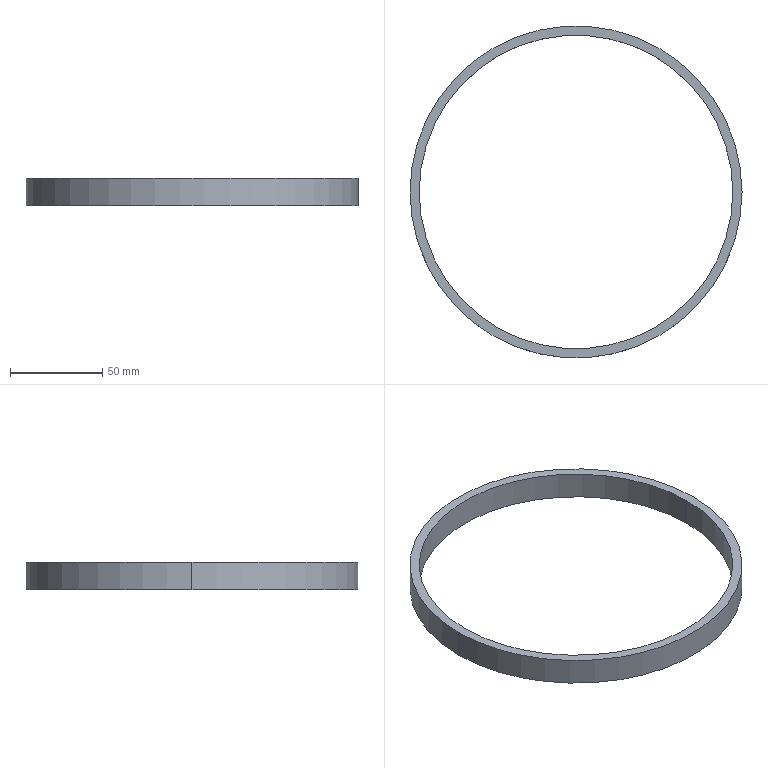Part | SolidWorks | features Extrusion 1 | 1 solid | 6 faces | box 180 x 180 x 15 mm | volume 41233 mm3 | cylinder 4 | plane 2 | commonest cylinder face diameters 170 x2 180 x2
STEP:
#1=CARTESIAN_POINT('',(-85.,0.,15.));
#2=VERTEX_POINT('',#1);
#3=CARTESIAN_POINT('',(85.,0.,15.));
#4=VERTEX_POINT('',#3);
#5=CARTESIAN_POINT('',(0.,0.,15.));
#6=DIRECTION('',(0.,0.,1.));
#7=DIRECTION('',(1.,0.,0.));
#8=AXIS2_PLACEMENT_3D('',#5,#6,#7);
#9=CIRCLE('',#8,85.);
#10=EDGE_CURVE('',#2,#4,#9,.T.);
#11=ORIENTED_EDGE('',*,*,#10,.T.);
#12=CARTESIAN_POINT('',(85.,0.,0.));
#13=VERTEX_POINT('',#12);
#14=CARTESIAN_POINT('',(85.,0.,15.));
#15=DIRECTION('',(0.,0.,-1.));
#16=VECTOR('',#15,1000.);
#17=LINE('',#14,#16);
#18=EDGE_CURVE('',#4,#13,#17,.T.);
#19=ORIENTED_EDGE('',*,*,#18,.T.);
#20=CARTESIAN_POINT('',(-85.,0.,0.));
#21=VERTEX_POINT('',#20);
#22=CARTESIAN_POINT('',(0.,0.,0.));
#23=DIRECTION('',(0.,0.,1.));
#24=DIRECTION('',(1.,0.,0.));
#25=AXIS2_PLACEMENT_3D('',#22,#23,#24);
#26=CIRCLE('',#25,85.);
#27=EDGE_CURVE('',#21,#13,#26,.T.);
#28=ORIENTED_EDGE('',*,*,#27,.F.);
#29=CARTESIAN_POINT('',(-85.,0.,15.));
#30=DIRECTION('',(0.,0.,-1.));
#31=VECTOR('',#30,1000.);
#32=LINE('',#29,#31);
#33=EDGE_CURVE('',#2,#21,#32,.T.);
#34=ORIENTED_EDGE('',*,*,#33,.F.);
#35=EDGE_LOOP('',(#11,#19,#28,#34));
#36=FACE_OUTER_BOUND('',#35,.T.);
#37=CARTESIAN_POINT('',(0.,0.,15.));
#38=DIRECTION('',(0.,0.,-1.));
#39=DIRECTION('',(-1.,0.,0.));
#40=AXIS2_PLACEMENT_3D('',#37,#38,#39);
#41=CYLINDRICAL_SURFACE('',#40,85.);
#42=ADVANCED_FACE('',(#36),#41,.F.);
#43=CARTESIAN_POINT('',(90.,0.,15.));
#44=VERTEX_POINT('',#43);
#45=CARTESIAN_POINT('',(-90.,0.,15.));
#46=VERTEX_POINT('',#45);
#47=CARTESIAN_POINT('',(0.,0.,15.));
#48=DIRECTION('',(0.,0.,1.));
#49=DIRECTION('',(1.,0.,0.));
#50=AXIS2_PLACEMENT_3D('',#47,#48,#49);
#51=CIRCLE('',#50,90.);
#52=EDGE_CURVE('',#44,#46,#51,.T.);
#53=ORIENTED_EDGE('',*,*,#52,.F.);
#54=CARTESIAN_POINT('',(90.,0.,0.));
#55=VERTEX_POINT('',#54);
#56=CARTESIAN_POINT('',(90.,0.,15.));
#57=DIRECTION('',(0.,0.,-1.));
#58=VECTOR('',#57,1000.);
#59=LINE('',#56,#58);
#60=EDGE_CURVE('',#44,#55,#59,.T.);
#61=ORIENTED_EDGE('',*,*,#60,.T.);
#62=CARTESIAN_POINT('',(-90.,0.,0.));
#63=VERTEX_POINT('',#62);
#64=CARTESIAN_POINT('',(0.,0.,0.));
#65=DIRECTION('',(0.,0.,1.));
#66=DIRECTION('',(1.,0.,0.));
#67=AXIS2_PLACEMENT_3D('',#64,#65,#66);
#68=CIRCLE('',#67,90.);
#69=EDGE_CURVE('',#55,#63,#68,.T.);
#70=ORIENTED_EDGE('',*,*,#69,.T.);
#71=CARTESIAN_POINT('',(-90.,0.,15.));
#72=DIRECTION('',(0.,0.,-1.));
#73=VECTOR('',#72,1000.);
#74=LINE('',#71,#73);
#75=EDGE_CURVE('',#46,#63,#74,.T.);
#76=ORIENTED_EDGE('',*,*,#75,.F.);
#77=EDGE_LOOP('',(#53,#61,#70,#76));
#78=FACE_OUTER_BOUND('',#77,.T.);
#79=CARTESIAN_POINT('',(0.,0.,15.));
#80=DIRECTION('',(0.,0.,-1.));
#81=DIRECTION('',(-1.,0.,0.));
#82=AXIS2_PLACEMENT_3D('',#79,#80,#81);
#83=CYLINDRICAL_SURFACE('',#82,90.);
#84=ADVANCED_FACE('',(#78),#83,.T.);
#85=CARTESIAN_POINT('',(0.,0.,15.));
#86=DIRECTION('',(0.,0.,1.));
#87=DIRECTION('',(1.,0.,0.));
#88=AXIS2_PLACEMENT_3D('',#85,#86,#87);
#89=CIRCLE('',#88,90.);
#90=EDGE_CURVE('',#46,#44,#89,.T.);
#91=ORIENTED_EDGE('',*,*,#90,.T.);
#92=ORIENTED_EDGE('',*,*,#52,.T.);
#93=EDGE_LOOP('',(#91,#92));
#94=FACE_OUTER_BOUND('',#93,.T.);
#95=ORIENTED_EDGE('',*,*,#10,.F.);
#96=CARTESIAN_POINT('',(0.,0.,15.));
#97=DIRECTION('',(0.,0.,1.));
#98=DIRECTION('',(1.,0.,0.));
#99=AXIS2_PLACEMENT_3D('',#96,#97,#98);
#100=CIRCLE('',#99,85.);
#101=EDGE_CURVE('',#4,#2,#100,.T.);
#102=ORIENTED_EDGE('',*,*,#101,.F.);
#103=EDGE_LOOP('',(#95,#102));
#104=FACE_BOUND('',#103,.T.);
#105=CARTESIAN_POINT('',(0.,0.,15.));
#106=DIRECTION('',(0.,0.,1.));
#107=DIRECTION('',(1.,0.,0.));
#108=AXIS2_PLACEMENT_3D('',#105,#106,#107);
#109=PLANE('',#108);
#110=ADVANCED_FACE('',(#94,#104),#109,.T.);
#111=CARTESIAN_POINT('',(0.,0.,0.));
#112=DIRECTION('',(0.,0.,1.));
#113=DIRECTION('',(1.,0.,0.));
#114=AXIS2_PLACEMENT_3D('',#111,#112,#113);
#115=CIRCLE('',#114,90.);
#116=EDGE_CURVE('',#63,#55,#115,.T.);
#117=ORIENTED_EDGE('',*,*,#116,.F.);
#118=ORIENTED_EDGE('',*,*,#69,.F.);
#119=EDGE_LOOP('',(#117,#118));
#120=FACE_OUTER_BOUND('',#119,.T.);
#121=ORIENTED_EDGE('',*,*,#27,.T.);
#122=CARTESIAN_POINT('',(0.,0.,0.));
#123=DIRECTION('',(0.,0.,1.));
#124=DIRECTION('',(1.,0.,0.));
#125=AXIS2_PLACEMENT_3D('',#122,#123,#124);
#126=CIRCLE('',#125,85.);
#127=EDGE_CURVE('',#13,#21,#126,.T.);
#128=ORIENTED_EDGE('',*,*,#127,.T.);
#129=EDGE_LOOP('',(#121,#128));
#130=FACE_BOUND('',#129,.T.);
#131=CARTESIAN_POINT('',(0.,0.,0.));
#132=DIRECTION('',(0.,0.,1.));
#133=DIRECTION('',(1.,0.,0.));
#134=AXIS2_PLACEMENT_3D('',#131,#132,#133);
#135=PLANE('',#134);
#136=ADVANCED_FACE('',(#120,#130),#135,.F.);
#137=ORIENTED_EDGE('',*,*,#60,.F.);
#138=ORIENTED_EDGE('',*,*,#90,.F.);
#139=ORIENTED_EDGE('',*,*,#75,.T.);
#140=ORIENTED_EDGE('',*,*,#116,.T.);
#141=EDGE_LOOP('',(#137,#138,#139,#140));
#142=FACE_OUTER_BOUND('',#141,.T.);
#143=CARTESIAN_POINT('',(0.,0.,15.));
#144=DIRECTION('',(0.,0.,-1.));
#145=DIRECTION('',(-1.,0.,0.));
#146=AXIS2_PLACEMENT_3D('',#143,#144,#145);
#147=CYLINDRICAL_SURFACE('',#146,90.);
#148=ADVANCED_FACE('',(#142),#147,.T.);
#149=ORIENTED_EDGE('',*,*,#18,.F.);
#150=ORIENTED_EDGE('',*,*,#101,.T.);
#151=ORIENTED_EDGE('',*,*,#33,.T.);
#152=ORIENTED_EDGE('',*,*,#127,.F.);
#153=EDGE_LOOP('',(#149,#150,#151,#152));
#154=FACE_OUTER_BOUND('',#153,.T.);
#155=CARTESIAN_POINT('',(0.,0.,15.));
#156=DIRECTION('',(0.,0.,-1.));
#157=DIRECTION('',(-1.,0.,0.));
#158=AXIS2_PLACEMENT_3D('',#155,#156,#157);
#159=CYLINDRICAL_SURFACE('',#158,85.);
#160=ADVANCED_FACE('',(#154),#159,.F.);
#161=CLOSED_SHELL('',(#42,#84,#110,#136,#148,#160));
#162=MANIFOLD_SOLID_BREP('',#161);
#163=CARTESIAN_POINT('',(0.,0.,0.));
#164=DIRECTION('',(0.,0.,1.));
#165=DIRECTION('',(1.,0.,0.));
#166=AXIS2_PLACEMENT_3D('',#163,#164,#165);
#167=(LENGTH_UNIT()NAMED_UNIT(*)SI_UNIT(.MILLI.,.METRE.));
#168=UNCERTAINTY_MEASURE_WITH_UNIT(LENGTH_MEASURE(0.00001),#167,'','');
#169=(NAMED_UNIT(*)PLANE_ANGLE_UNIT()SI_UNIT($,.RADIAN.));
#170=(NAMED_UNIT(*)SI_UNIT($,.STERADIAN.)SOLID_ANGLE_UNIT());
#171=(GEOMETRIC_REPRESENTATION_CONTEXT(3)GLOBAL_UNCERTAINTY_ASSIGNED_CONTEXT((#168))GLOBAL_UNIT_ASSIGNED_CONTEXT((#167,#169,#170))REPRESENTATION_CONTEXT('',''));
#172=ADVANCED_BREP_SHAPE_REPRESENTATION('',(#162,#166),#171);